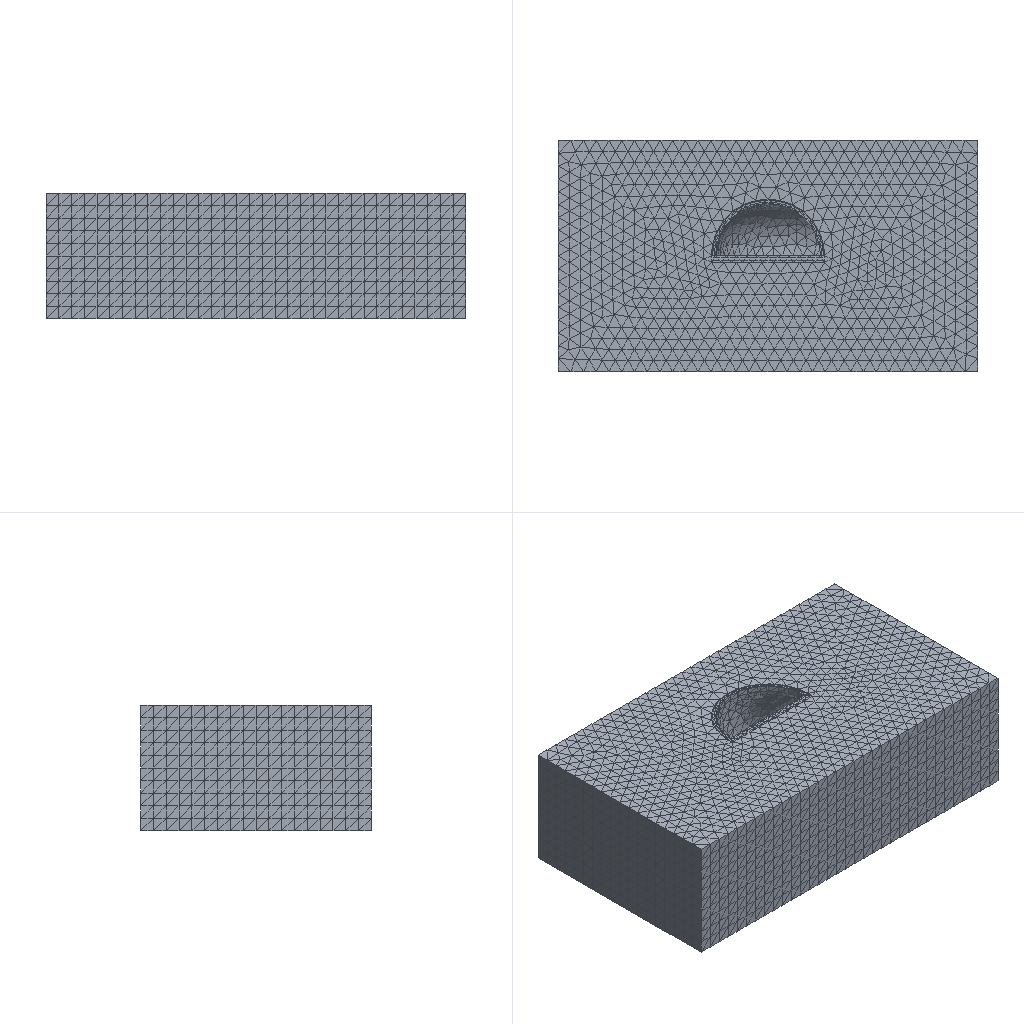Simulation study | abaqus
Set-up summary:
category,name,step,type,value,unit,region
solver,abaqus
solver,version,,,Abaqus/Standard 2020
units,not stated in the deck,,not stated
analysis,deck,,static,static
load_step,Step-1,Step-1,static
load_step,requested,,,1
mesh,nodes,,,68040
mesh,elements,,,45156
element_type,S4R,,shell,3336
element_type,C3D10,,solid,41820
load,load commands in deck,,count,2
bc,support commands in deck,,count,3
material,CONCRETE,,in results
material,REBAR,,in results
material,SOIL,,in results
check,setup vs results,,match,"per instance, exact: element labels, types and connectivity; labels of the nodes the elements use; coordinates of those nodes at SINGLE_PRECISION in 2 of 4 instance(s)"
Abaqus input file, long lists of numbers shortened:
*Heading
** Job name: Job-2 Model name: Model-1-Copy
** Generated by: Abaqus/CAE 2020
*Preprint, echo=NO, model=NO, history=NO, contact=NO
**
** PARTS
**
*Part, name=Part-1
*Node
      1,         -10.,          -4.,           6.
      2,         -10.,           7.,           6.
** (55328 more lines like these left out)
*Element, type=C3D10
    1,  2809,  2810,  2811,  2812,  7627,  7626,  7625,  7629,  7628,  7630
    2,  2809,  2810,  2813,  2814,  7627,  7632,  7631,  7634,  7633,  7635
** (37272 more lines like these left out)
*Nset, nset=Set-11, generate
     1,  55330,      1
*Elset, elset=Set-11, generate
     1,  37274,      1
** Section: Section-1-soil
*Solid Section, elset=Set-11, material=soil
,
*End Part
**
*Part, name=con
*Node
      1,   14.217,   1.55,           0.
      2,   14.217,   6.95,           0.
** (9141 more lines like these left out)
*Element, type=C3D10
   1, 1514,   19, 1299,    4, 1545, 1544, 1543, 1547, 1546, 1548
   2, 1514,   18,   19,    4, 1550, 1549, 1545, 1547, 1551, 1546
** (4544 more lines like these left out)
*Nset, nset=Set-5, generate
    1,  9143,     1
*Elset, elset=Set-5, generate
    1,  4546,     1
** Section: Section-2-concrete
*Solid Section, elset=Set-5, material=concrete
,
*End Part
**
*Part, name=jin-zhixian
*Node
      1,   14.37,   1.487, -0.215
      2,   14.37,    6.702, -0.215
** (1070 more lines like these left out)
*Element, type=S4R
  1,   1,  17, 237,  78
  2,  17,  18, 238, 237
** (976 more lines like these left out)
*Nset, nset=Set-1, generate
    1,  1072,     1
*Elset, elset=Set-1, generate
   1,  978,    1
** Section: rebar
*Shell Section, elset=Set-1, material=rebar
0.001, 5
*End Part
**
*Part, name=xian-wanqu
*Node
      1,   12.382,   8.64,           0.
      2,   12.382,   3.53,           0.
** (2493 more lines like these left out)
*Element, type=S4R
  1,   1,  17, 377, 114
  2,  17,  18, 378, 377
** (2356 more lines like these left out)
*Nset, nset=Set-1, generate
    1,  2495,     1
*Elset, elset=Set-1, generate
    1,  2358,     1
** Section: rebar
*Shell Section, elset=Set-1, material=rebar
0.001, 5
*End Part
**
**
** ASSEMBLY
**
*Assembly, name=Assembly
**
*Instance, name=Part-1-1, part=Part-1
*End Instance
**
*Instance, name=con-1, part=con
    -4.217,          1.5,     7.25
    -4.217,          1.5,     7.25, -5.217,          1.5,     7.25, 90.
*End Instance
**
*Instance, name=xian-wanqu-1, part=xian-wanqu
   -2.382,          1.5,      9.085
   -2.382,          1.5,      9.085, -3.382,          1.5,      9.085, 90.
*End Instance
**
*Instance, name=jin-zhixian-1, part=jin-zhixian
   -4.373,        1.505,     7.097
   -4.373,        1.505,     7.097, -5.373,        1.505,     7.097, 90.
*End Instance
**
*Nset, nset=Set-12, instance=Part-1-1
     1,     2,     3,     4,     7,     8,    10,    13,    15,    16,    17,    18,    23,    24,    25,    26
    27,    28,    29,    30,    31,    32,    33,    34,    35,    36,    37,    38,    39,    49,    50,    51
** (330 more lines like these left out)
*Nset, nset=Set-12, instance=con-1
   15,   16,   17,   18,   21,   22,  246,  247,  248,  249,  250,  251,  252,  253,  254,  255
  256,  257,  258,  259,  260,  261,  262,  263,  264,  265,  266,  267,  268,  269,  270,  271
** (9 more lines like these left out)
*Elset, elset=Set-12, instance=Part-1-1
   434,   722,  1164,  1419,  1428,  1433,  1450,  1775,  2163,  2497,  2633,  2863,  3012,  3375,  3883,  3886
  3887,  3897,  3910,  3912,  3933,  3971,  3973,  3976,  3983,  3984,  3991,  4027,  4034,  4045,  4068,  4078
** (157 more lines like these left out)
*Elset, elset=Set-12, instance=con-1
   40,   49,   57,   59,  274,  415,  552,  553,  558,  559,  561,  567,  568,  570,  571,  574
  575,  584,  590,  903, 1012, 1014, 1044, 1057, 1064, 1133, 1141, 1231, 1233, 1284, 1372, 1718
** (2 more lines like these left out)
*Nset, nset=Set-13, instance=Part-1-1
     1,     2,     3,     4,    15,    16,    17,    18,    19,    20,    21,    22,    23,    24,    25,    26
    27,    28,    29,    30,    31,    32,    33,    34,    35,    36,    37,    38,    39,    40,    41,    42
** (93 more lines like these left out)
*Nset, nset=Set-13, instance=con-1
    1,    2,    5,    7,   11,   12,   23,   24,   25,   26,   27,   28,   29,   30,   31,   32
   33,   34,   35,   36,   37,   38,   97,   98,   99,  100,  101,  102,  103,  104,  105,  106
** (9 more lines like these left out)
*Elset, elset=Set-13, instance=Part-1-1
    23,    27,    33,   105,   114,   162,   185,   222,   240,   250,   277,   278,   281,   325,   340,   348
   357,   376,   399,   445,   479,   531,   610,   617,   629,   661,   664,   695,   696,   698,   715,   720
** (42 more lines like these left out)
*Elset, elset=Set-13, instance=con-1
   15,  151,  603,  606,  985,  992, 1759, 1763, 1768, 1774, 1842, 1893, 1929, 1949, 1989, 1995
 2027, 2083, 2190, 2207, 3156, 3243, 3245, 3246, 3257, 3264, 3267, 3271, 3289, 3310, 3337, 3350
** (2 more lines like these left out)
*Nset, nset=Set-14, instance=Part-1-1
     1,     4,    17,    18,    66,    67,    68,    69,    70,    71,    72,    73,    74,   229,   230,   231
   232,   233,   234,   235,   236,   237,   238,   239,   240,   241,   242,   243,   244,   245,   246,   247
** (86 more lines like these left out)
*Elset, elset=Set-14, instance=Part-1-1
    69,   397,   434,   865,  1488,  1601,  1758,  1978,  2271,  2398,  3908,  3941,  4089,  4188,  4191,  4192
  4197,  4222,  4224,  4230,  4232,  4241,  4311,  4314,  4315,  4444,  4446,  4480,  4532,  4704,  4788,  4899
** (40 more lines like these left out)
*Nset, nset=Set-17, instance=Part-1-1, generate
     1,  55330,      1
*Elset, elset=Set-17, instance=Part-1-1, generate
     1,  37274,      1
*Nset, nset=m_Set-10, instance=xian-wanqu-1, generate
    1,  2495,     1
*Elset, elset=m_Set-10, instance=xian-wanqu-1, generate
    1,  2358,     1
*Nset, nset=m_Set-15, instance=jin-zhixian-1, generate
    1,  1072,     1
*Elset, elset=m_Set-15, instance=jin-zhixian-1, generate
   1,  978,    1
*Nset, nset=s_Set-10, instance=con-1, generate
    1,  9143,     1
*Elset, elset=s_Set-10, instance=con-1, generate
    1,  4546,     1
*Nset, nset=s_Set-15, instance=con-1, generate
    1,  9143,     1
*Elset, elset=s_Set-15, instance=con-1, generate
    1,  4546,     1
*Elset, elset=_Surf-4_S2, internal, instance=Part-1-1
    28,  3949,  4042,  4879,  6136,  6727,  6736,  6778,  6912,  7016, 15970, 16785, 24559
*Elset, elset=_Surf-4_S4, internal, instance=Part-1-1
   150,  4682,  5415,  6774,  7453,  7537, 10701, 11663, 11828, 13350, 13518, 13706, 13823, 16380, 19620, 19834
 19958, 21048, 21795, 27464, 32811
*Elset, elset=_Surf-4_S3, internal, instance=Part-1-1
   496,   626,  2450,  2460,  2631,  2708,  3965,  3976,  3991,  4025,  4045,  4048,  4054,  4154,  4178,  4248
  4249,  4253,  4272,  4286,  4322,  4341,  4362,  4371,  4684,  4776,  4848,  4852,  4855,  4872,  4943,  5122
** (36 more lines like these left out)
*Elset, elset=_Surf-4_S1, internal, instance=Part-1-1
  4775,  6703,  6766,  6776,  6813,  6841,  6876,  6913,  6939,  6965,  6999, 13389, 13853, 13886, 17428, 17886
 20117, 20118, 20896, 28162
*Surface, type=ELEMENT, name=Surf-4
_Surf-4_S2, S2
_Surf-4_S4, S4
_Surf-4_S3, S3
_Surf-4_S1, S1
*Elset, elset=_m_Surf-2_S3, internal, instance=con-1
   16,   39,   56,   61,  111,  208,  210,  213,  219,  259,  263,  289,  291,  399,  403,  420
  453,  457,  514,  521,  522,  531,  556,  557,  573,  606,  621,  628,  651,  674,  677,  689
** (61 more lines like these left out)
*Elset, elset=_m_Surf-2_S2, internal, instance=con-1
   19,   21,   28,   41,   47,   54,   68,   90,   95,  127,  130,  149,  168,  257,  260,  267
  272,  275,  277,  285,  295,  583,  586,  633,  654,  657,  721,  731,  756,  759,  760,  794
** (13 more lines like these left out)
*Elset, elset=_m_Surf-2_S4, internal, instance=con-1
   75,   76,   96,  105,  144,  148,  162,  165,  189,  196,  206,  230,  251,  261,  264,  290
  293,  303,  537,  602,  631,  636,  637,  647,  683,  693,  708,  733,  736,  752,  783,  833
** (12 more lines like these left out)
*Elset, elset=_m_Surf-2_S1, internal, instance=con-1
    9,  101,  118,  158,  176,  198,  216,  222,  236,  249,  286,  297,  332,  402,  590,  656
  697,  753,  790,  802,  857,  923,  976,  984, 1102, 1110, 1178, 1209, 1227, 1241, 1275, 1396
** (8 more lines like these left out)
*Surface, type=ELEMENT, name=m_Surf-2
_m_Surf-2_S3, S3
_m_Surf-2_S2, S2
_m_Surf-2_S4, S4
_m_Surf-2_S1, S1
*Elset, elset=_s_Surf-2_S3, internal, instance=Part-1-1
   260,   977,  1349,  1414,  1602,  1741,  2984,  3978,  4003,  4040,  4081,  4093,  4102,  4145,  4153,  4243
  4254,  4256,  4263,  4276,  4290,  4293,  4307,  4331,  4337,  4369,  4419,  4425,  4429,  4430,  5553,  5557
** (54 more lines like these left out)
*Elset, elset=_s_Surf-2_S1, internal, instance=Part-1-1
  1393,  3987,  5630,  5661,  5705,  6543,  6557,  8583, 10066, 10352, 10706, 13988, 14295, 14607, 14631, 15377
 15909, 16978, 17020, 17021, 17184, 17228, 17238, 17271, 17283, 17298, 17302, 17312, 17323, 17334, 17353, 17356
** (3 more lines like these left out)
*Elset, elset=_s_Surf-2_S4, internal, instance=Part-1-1
  4373,  5586,  5590,  5666,  5714,  5715,  5861,  5999,  6334,  6381,  7966,  8416,  9873, 10007, 10175, 10221
 10560, 13997, 14024, 17216, 17235, 17245, 17262, 17274, 17284, 17297, 17311, 17331, 17340, 17351, 17360, 17390
** (3 more lines like these left out)
*Elset, elset=_s_Surf-2_S2, internal, instance=Part-1-1
  1909,  3982,  4397,  5874,  6236,  6434,  8316,  9395,  9991, 10363, 10372, 10694, 10723, 10756, 13872, 14018
 14575, 15900, 16121, 17246, 17263, 17265, 17344, 17422, 17474, 17626, 17628, 17695, 17715, 17798, 17873, 17949
** (1 more lines like these left out)
*Surface, type=ELEMENT, name=s_Surf-2
_s_Surf-2_S3, S3
_s_Surf-2_S1, S1
_s_Surf-2_S4, S4
_s_Surf-2_S2, S2
** Constraint: Constraint-1
*Embedded Element, host elset=s_Set-10
m_Set-10
** Constraint: Constraint-2
*Tie, name=Constraint-2, adjust=yes
s_Surf-2, m_Surf-2
** Constraint: Constraint-3
*Embedded Element, host elset=s_Set-15
m_Set-15
*End Assembly
*Amplitude, name=Amp-1
             0.,              0.,              1.,              1.
**
** MATERIALS
**
*Material, name=concrete
*Density
2500.,
*Elastic
 2.9791e+10, 0.2
*Concrete Damaged Plasticity
30.,    0.1,   1.16, 0.6667,   0.05
*Concrete Compression Hardening
 1.54e+07,      0.
 1.69e+07,  0.0002
 1.96e+07, 0.00048
 2.01e+07, 0.00079
    2e+07, 0.00095
 1.96e+07,  0.0011
 1.91e+07, 0.00127
 1.86e+07, 0.00143
 1.79e+07,  0.0016
 1.72e+07, 0.00177
 1.66e+07, 0.00194
 1.59e+07, 0.00211
 1.53e+07, 0.00228
 1.47e+07, 0.00245
 1.41e+07, 0.00261
 1.35e+07, 0.00278
  1.3e+07, 0.00294
 1.25e+07,  0.0031
  1.2e+07, 0.00327
 1.16e+07, 0.00343
 1.12e+07, 0.00359
 1.08e+07, 0.00375
 1.04e+07, 0.00391
 1.01e+07, 0.00406
*Concrete Tension Stiffening
 2.06e+06,      0.
 1.92e+06,   2e-05
 1.72e+06,   4e-05
 1.53e+06,   6e-05
 1.37e+06,   8e-05
 1.24e+06,  0.0001
 1.13e+06, 0.00011
 1.04e+06, 0.00013
  970000., 0.00015
  900000., 0.00016
  850000., 0.00018
*Concrete Compression Damage
     0.,      0.
 0.0841,   9e-05
 0.0933,  0.0001
 0.1091, 0.00013
 0.1418,  0.0002
 0.2407, 0.00048
  0.322, 0.00079
 0.3557, 0.00095
 0.3886,  0.0011
 0.4201, 0.00127
 0.4499, 0.00143
 0.4778,  0.0016
 0.5039, 0.00177
 0.5282, 0.00194
 0.5506, 0.00211
 0.5715, 0.00228
 0.5908, 0.00245
 0.6086, 0.00261
 0.6252, 0.00278
 0.6406, 0.00294
 0.6549,  0.0031
 0.6682, 0.00327
 0.6806, 0.00343
 0.6922, 0.00359
  0.703, 0.00375
 0.7131, 0.00391
 0.7227, 0.00406
   0.74, 0.00438
 0.7554, 0.00469
 0.7691,   0.005
 0.7815, 0.00531
 0.7926, 0.00561
 0.8026, 0.00592
 0.8118, 0.00622
 0.8202, 0.00653
 0.8278, 0.00683
 0.8349, 0.00713
*Concrete Tension Damage
      0.,      0.
 0.1181,   2e-05
 0.2281,   4e-05
 0.3187,   6e-05
 0.3919,   8e-05
 0.4512,  0.0001
 0.5, 0.00011
  0.5407, 0.00013
 0.575, 0.00015
 0.6043, 0.00016
 0.6297, 0.00018
 0.7177, 0.00025
 0.7702, 0.00033
 0.8053,  0.0004
 0.8304, 0.00047
 0.8494, 0.00054
  0.8643, 0.00061
 0.8763, 0.00068
 0.8862, 0.00075
*Material, name=rebar
*Density
7860.,
*Elastic
 2.1e+11, 0.3
*Material, name=soil
*Density
1800.,
*Elastic
 4.79e+07, 0.35
*Mohr Coulomb
25.,0.
*Mohr Coulomb Hardening
25000.,0.
**
** PREDEFINED FIELDS
**
** Name: Predefined Field-1   Type: Geostatic stress
*Initial Conditions, type=STRESS, GEOSTATIC
Set-17, 0., 6., -20000., -4., 2., 2.
** ----------------------------------------------------------------
**
** STEP: Step-1
**
*Step, name=Step-1, nlgeom=YES, inc=1000
*Static, stabilize=0.0002, allsdtol=0.05, continue=NO
0.01, 1., 1e-05, 1.
**
** BOUNDARY CONDITIONS
**
** Name: BC-1 Type: 位移/转角
*Boundary
Set-12, 3, 3
** Name: BC-2 Type: 位移/转角
*Boundary
Set-13, 1, 1
** Name: BC-3 Type: 位移/转角
*Boundary
Set-14, 2, 2
**
** LOADS
**
** Name: Load-2   Type: Pressure
*Dsload, amplitude=Amp-1
Surf-4, P, 1e+06
** Name: Load-3   Type: Gravity
*Dload
, GRAV, 9.8, 0., -1., 0.
**
** OUTPUT REQUESTS
**
*Restart, write, frequency=0
**
** FIELD OUTPUT: F-Output-1
**
*Output, field
*Node Output
CF, RF, RM, RT, TF, U, V
*Element Output, directions=YES
DAMAGEC, DAMAGET, E, LE, MISES, MISESMAX, PE, PEEQ, PEMAG, S, SDEG, SF, SSAVG
*Contact Output
CDISP, CSTRESS
**
** HISTORY OUTPUT: H-Output-1
**
*Output, history, variable=PRESELECT
*End Step
Results summary:
result,step,,partial,increments=17 time=0.4931/1.0
result,analysis,,,static
result,last_loadstep,,,1
result,primary field,,,"U, UR"
result,reaction total,,FX,34757.305,model units
result,reaction total,,FY,69644021.468,model units
result,reaction total,,FZ,16239.463,model units